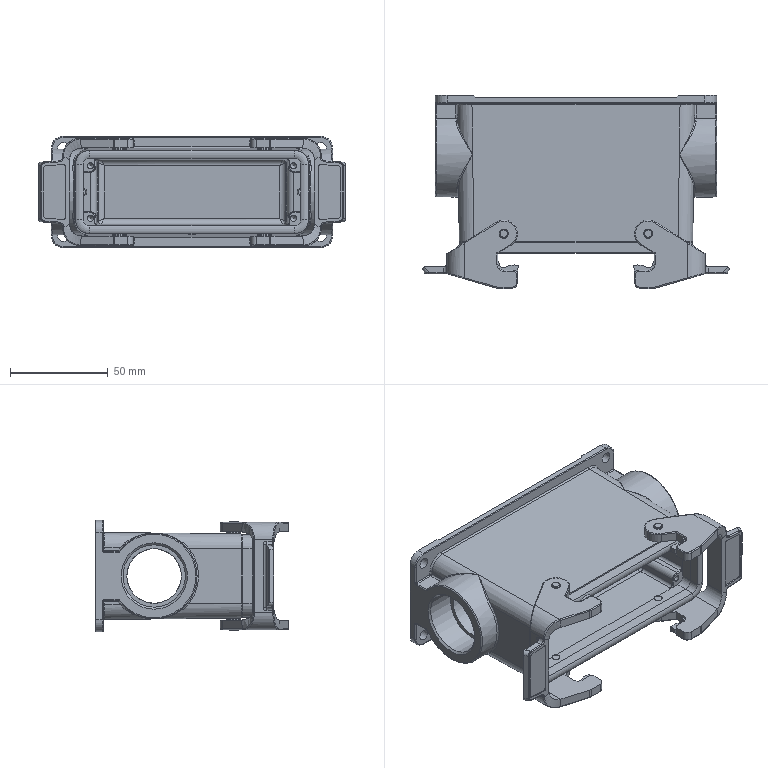Part | NX | features BREP 3 | 3 solids | 689 faces | box 157.408 x 98.8 x 57 mm | volume 183143 mm3 | plane 264 | cylinder 257 | spline 92 | torus 58 | cone 18 | commonest cylinder face diameters 1 x80 6 x26 4 x18 3 x16 14 x12 44.6 x11